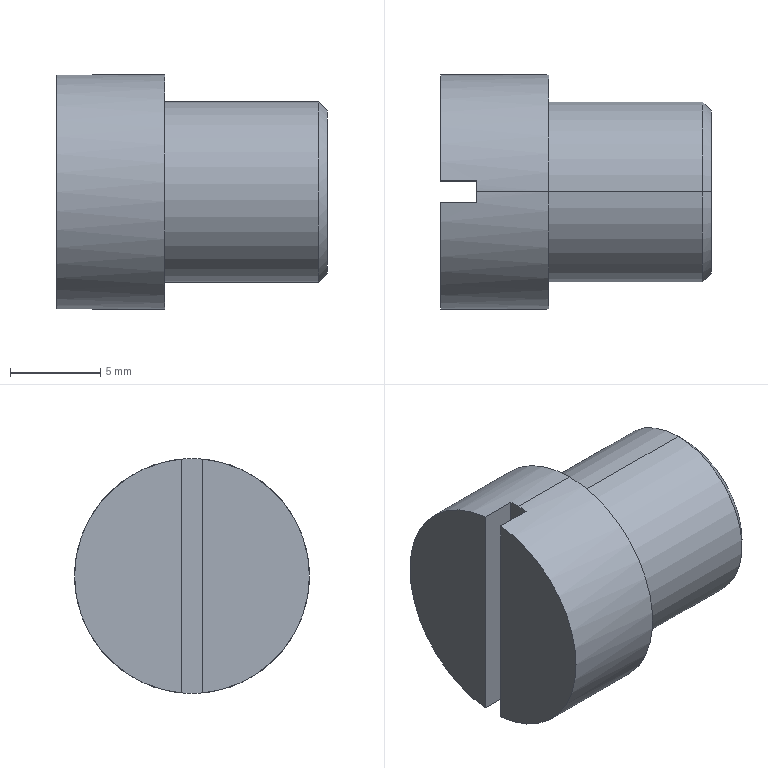Part | SolidWorks | features ICE 2, 3DProfileFeature 1, Chamfer 1, Extrusion 1, HoleWzd 1 | 1 solid | 17 faces | box 15 x 13 x 13 mm | volume 1310 mm3 | plane 7 | cylinder 6 | cone 4 | commonest cylinder face diameters 4.2 x2 10 x2 13 x2
STEP:
#1=CARTESIAN_POINT('',(9.,0.,-4.5));
#2=VERTEX_POINT('',#1);
#3=CARTESIAN_POINT('',(9.,0.,4.5));
#4=VERTEX_POINT('',#3);
#5=CARTESIAN_POINT('',(9.,0.,0.));
#6=DIRECTION('',(1.,0.,0.));
#7=DIRECTION('',(0.,0.,-1.));
#8=AXIS2_PLACEMENT_3D('',#5,#6,#7);
#9=CIRCLE('',#8,4.5);
#10=EDGE_CURVE('',#2,#4,#9,.T.);
#11=ORIENTED_EDGE('',*,*,#10,.F.);
#12=CARTESIAN_POINT('',(8.5,0.,-5.));
#13=VERTEX_POINT('',#12);
#14=CARTESIAN_POINT('',(9.,0.,-4.5));
#15=DIRECTION('',(-0.7071,0.,-0.7071));
#16=VECTOR('',#15,1000.);
#17=LINE('',#14,#16);
#18=EDGE_CURVE('',#2,#13,#17,.T.);
#19=ORIENTED_EDGE('',*,*,#18,.T.);
#20=CARTESIAN_POINT('',(8.5,0.,5.));
#21=VERTEX_POINT('',#20);
#22=CARTESIAN_POINT('',(8.5,0.,0.));
#23=DIRECTION('',(-1.,0.,0.));
#24=DIRECTION('',(0.,0.,-1.));
#25=AXIS2_PLACEMENT_3D('',#22,#23,#24);
#26=CIRCLE('',#25,5.);
#27=EDGE_CURVE('',#21,#13,#26,.T.);
#28=ORIENTED_EDGE('',*,*,#27,.F.);
#29=CARTESIAN_POINT('',(9.,0.,4.5));
#30=DIRECTION('',(-0.7071,0.,0.7071));
#31=VECTOR('',#30,1000.);
#32=LINE('',#29,#31);
#33=EDGE_CURVE('',#4,#21,#32,.T.);
#34=ORIENTED_EDGE('',*,*,#33,.F.);
#35=EDGE_LOOP('',(#11,#19,#28,#34));
#36=FACE_OUTER_BOUND('',#35,.T.);
#37=CARTESIAN_POINT('',(9.,0.,0.));
#38=DIRECTION('',(-1.,0.,0.));
#39=DIRECTION('',(0.,0.,1.));
#40=AXIS2_PLACEMENT_3D('',#37,#38,#39);
#41=CONICAL_SURFACE('',#40,4.5,0.7854);
#42=ADVANCED_FACE('',(#36),#41,.T.);
#43=CARTESIAN_POINT('',(-2.,0.,2.1));
#44=VERTEX_POINT('',#43);
#45=CARTESIAN_POINT('',(-2.,0.,-2.1));
#46=VERTEX_POINT('',#45);
#47=CARTESIAN_POINT('',(-2.,0.,0.));
#48=DIRECTION('',(1.,0.,0.));
#49=DIRECTION('',(0.,0.,-1.));
#50=AXIS2_PLACEMENT_3D('',#47,#48,#49);
#51=CIRCLE('',#50,2.1);
#52=EDGE_CURVE('',#44,#46,#51,.T.);
#53=ORIENTED_EDGE('',*,*,#52,.F.);
#54=CARTESIAN_POINT('',(9.,0.,2.1));
#55=VERTEX_POINT('',#54);
#56=CARTESIAN_POINT('',(9.,0.,2.1));
#57=DIRECTION('',(1.,0.,0.));
#58=VECTOR('',#57,1000.);
#59=LINE('',#56,#58);
#60=EDGE_CURVE('',#44,#55,#59,.T.);
#61=ORIENTED_EDGE('',*,*,#60,.T.);
#62=CARTESIAN_POINT('',(9.,0.,-2.1));
#63=VERTEX_POINT('',#62);
#64=CARTESIAN_POINT('',(9.,0.,0.));
#65=DIRECTION('',(1.,0.,0.));
#66=DIRECTION('',(0.,0.,-1.));
#67=AXIS2_PLACEMENT_3D('',#64,#65,#66);
#68=CIRCLE('',#67,2.1);
#69=EDGE_CURVE('',#55,#63,#68,.T.);
#70=ORIENTED_EDGE('',*,*,#69,.T.);
#71=CARTESIAN_POINT('',(9.,0.,-2.1));
#72=DIRECTION('',(1.,0.,0.));
#73=VECTOR('',#72,1000.);
#74=LINE('',#71,#73);
#75=EDGE_CURVE('',#46,#63,#74,.T.);
#76=ORIENTED_EDGE('',*,*,#75,.F.);
#77=EDGE_LOOP('',(#53,#61,#70,#76));
#78=FACE_OUTER_BOUND('',#77,.T.);
#79=CARTESIAN_POINT('',(9.,0.,0.));
#80=DIRECTION('',(1.,0.,0.));
#81=DIRECTION('',(0.,0.,-1.));
#82=AXIS2_PLACEMENT_3D('',#79,#80,#81);
#83=CYLINDRICAL_SURFACE('',#82,2.1);
#84=ADVANCED_FACE('',(#78),#83,.F.);
#85=CARTESIAN_POINT('',(-3.262,0.,0.));
#86=VERTEX_POINT('',#85);
#87=CARTESIAN_POINT('',(-2.,0.,-2.1));
#88=DIRECTION('',(0.515,0.,-0.8572));
#89=VECTOR('',#88,1000.);
#90=LINE('',#87,#89);
#91=EDGE_CURVE('',#86,#46,#90,.T.);
#92=ORIENTED_EDGE('',*,*,#91,.F.);
#93=CARTESIAN_POINT('',(-2.,0.,2.1));
#94=DIRECTION('',(0.515,0.,0.8572));
#95=VECTOR('',#94,1000.);
#96=LINE('',#93,#95);
#97=EDGE_CURVE('',#86,#44,#96,.T.);
#98=ORIENTED_EDGE('',*,*,#97,.T.);
#99=ORIENTED_EDGE('',*,*,#52,.T.);
#100=EDGE_LOOP('',(#92,#98,#99));
#101=FACE_OUTER_BOUND('',#100,.T.);
#102=CARTESIAN_POINT('',(-2.,0.,0.));
#103=DIRECTION('',(1.,0.,0.));
#104=DIRECTION('',(0.,0.,-1.));
#105=AXIS2_PLACEMENT_3D('',#102,#103,#104);
#106=CONICAL_SURFACE('',#105,2.1,1.03);
#107=ADVANCED_FACE('',(#101),#106,.F.);
#108=CARTESIAN_POINT('',(-4.,0.,6.5));
#109=VERTEX_POINT('',#108);
#110=CARTESIAN_POINT('',(-4.,0.6,6.472));
#111=VERTEX_POINT('',#110);
#112=CARTESIAN_POINT('',(-4.,0.,0.));
#113=DIRECTION('',(-1.,0.,0.));
#114=DIRECTION('',(0.,0.,1.));
#115=AXIS2_PLACEMENT_3D('',#112,#113,#114);
#116=CIRCLE('',#115,6.5);
#117=EDGE_CURVE('',#109,#111,#116,.T.);
#118=ORIENTED_EDGE('',*,*,#117,.F.);
#119=CARTESIAN_POINT('',(0.,0.,6.5));
#120=VERTEX_POINT('',#119);
#121=CARTESIAN_POINT('',(-6.,0.,6.5));
#122=DIRECTION('',(1.,0.,0.));
#123=VECTOR('',#122,1000.);
#124=LINE('',#121,#123);
#125=EDGE_CURVE('',#109,#120,#124,.T.);
#126=ORIENTED_EDGE('',*,*,#125,.T.);
#127=CARTESIAN_POINT('',(0.,0.,-6.5));
#128=VERTEX_POINT('',#127);
#129=CARTESIAN_POINT('',(0.,0.,0.));
#130=DIRECTION('',(-1.,0.,0.));
#131=DIRECTION('',(0.,0.,1.));
#132=AXIS2_PLACEMENT_3D('',#129,#130,#131);
#133=CIRCLE('',#132,6.5);
#134=EDGE_CURVE('',#120,#128,#133,.T.);
#135=ORIENTED_EDGE('',*,*,#134,.T.);
#136=CARTESIAN_POINT('',(-4.,0.,-6.5));
#137=VERTEX_POINT('',#136);
#138=CARTESIAN_POINT('',(-6.,0.,-6.5));
#139=DIRECTION('',(1.,0.,0.));
#140=VECTOR('',#139,1000.);
#141=LINE('',#138,#140);
#142=EDGE_CURVE('',#137,#128,#141,.T.);
#143=ORIENTED_EDGE('',*,*,#142,.F.);
#144=CARTESIAN_POINT('',(-4.,0.6,-6.472));
#145=VERTEX_POINT('',#144);
#146=CARTESIAN_POINT('',(-4.,0.,0.));
#147=DIRECTION('',(-1.,0.,0.));
#148=DIRECTION('',(0.,0.,1.));
#149=AXIS2_PLACEMENT_3D('',#146,#147,#148);
#150=CIRCLE('',#149,6.5);
#151=EDGE_CURVE('',#145,#137,#150,.T.);
#152=ORIENTED_EDGE('',*,*,#151,.F.);
#153=CARTESIAN_POINT('',(-6.,0.6,-6.472));
#154=VERTEX_POINT('',#153);
#155=CARTESIAN_POINT('',(-6.,0.6,-6.472));
#156=DIRECTION('',(-1.,0.,0.));
#157=VECTOR('',#156,1000.);
#158=LINE('',#155,#157);
#159=EDGE_CURVE('',#145,#154,#158,.T.);
#160=ORIENTED_EDGE('',*,*,#159,.T.);
#161=CARTESIAN_POINT('',(-6.,0.6,6.472));
#162=VERTEX_POINT('',#161);
#163=CARTESIAN_POINT('',(-6.,0.,0.));
#164=DIRECTION('',(-1.,0.,0.));
#165=DIRECTION('',(0.,0.,1.));
#166=AXIS2_PLACEMENT_3D('',#163,#164,#165);
#167=CIRCLE('',#166,6.5);
#168=EDGE_CURVE('',#162,#154,#167,.T.);
#169=ORIENTED_EDGE('',*,*,#168,.F.);
#170=CARTESIAN_POINT('',(-6.,0.6,6.472));
#171=DIRECTION('',(1.,0.,0.));
#172=VECTOR('',#171,1000.);
#173=LINE('',#170,#172);
#174=EDGE_CURVE('',#162,#111,#173,.T.);
#175=ORIENTED_EDGE('',*,*,#174,.T.);
#176=EDGE_LOOP('',(#118,#126,#135,#143,#152,#160,#169,#175));
#177=FACE_OUTER_BOUND('',#176,.T.);
#178=CARTESIAN_POINT('',(-6.,0.,0.));
#179=DIRECTION('',(1.,0.,0.));
#180=DIRECTION('',(0.,0.,-1.));
#181=AXIS2_PLACEMENT_3D('',#178,#179,#180);
#182=CYLINDRICAL_SURFACE('',#181,6.5);
#183=ADVANCED_FACE('',(#177),#182,.T.);
#184=ORIENTED_EDGE('',*,*,#27,.T.);
#185=CARTESIAN_POINT('',(0.,0.,-5.));
#186=VERTEX_POINT('',#185);
#187=CARTESIAN_POINT('',(9.,0.,-5.));
#188=DIRECTION('',(-1.,0.,0.));
#189=VECTOR('',#188,1000.);
#190=LINE('',#187,#189);
#191=EDGE_CURVE('',#13,#186,#190,.T.);
#192=ORIENTED_EDGE('',*,*,#191,.T.);
#193=CARTESIAN_POINT('',(0.,0.,5.));
#194=VERTEX_POINT('',#193);
#195=CARTESIAN_POINT('',(0.,0.,0.));
#196=DIRECTION('',(-1.,0.,0.));
#197=DIRECTION('',(0.,0.,1.));
#198=AXIS2_PLACEMENT_3D('',#195,#196,#197);
#199=CIRCLE('',#198,5.);
#200=EDGE_CURVE('',#194,#186,#199,.T.);
#201=ORIENTED_EDGE('',*,*,#200,.F.);
#202=CARTESIAN_POINT('',(9.,0.,5.));
#203=DIRECTION('',(-1.,0.,0.));
#204=VECTOR('',#203,1000.);
#205=LINE('',#202,#204);
#206=EDGE_CURVE('',#21,#194,#205,.T.);
#207=ORIENTED_EDGE('',*,*,#206,.F.);
#208=EDGE_LOOP('',(#184,#192,#201,#207));
#209=FACE_OUTER_BOUND('',#208,.T.);
#210=CARTESIAN_POINT('',(9.,0.,0.));
#211=DIRECTION('',(-1.,0.,0.));
#212=DIRECTION('',(0.,0.,1.));
#213=AXIS2_PLACEMENT_3D('',#210,#211,#212);
#214=CYLINDRICAL_SURFACE('',#213,5.);
#215=ADVANCED_FACE('',(#209),#214,.T.);
#216=CARTESIAN_POINT('',(-6.,-0.6,-6.472));
#217=VERTEX_POINT('',#216);
#218=CARTESIAN_POINT('',(-6.,-0.6,6.472));
#219=VERTEX_POINT('',#218);
#220=CARTESIAN_POINT('',(-6.,-0.6,0.));
#221=DIRECTION('',(0.,0.,1.));
#222=VECTOR('',#221,1000.);
#223=LINE('',#220,#222);
#224=EDGE_CURVE('',#217,#219,#223,.T.);
#225=ORIENTED_EDGE('',*,*,#224,.F.);
#226=CARTESIAN_POINT('',(-6.,0.,0.));
#227=DIRECTION('',(-1.,0.,0.));
#228=DIRECTION('',(0.,0.,1.));
#229=AXIS2_PLACEMENT_3D('',#226,#227,#228);
#230=CIRCLE('',#229,6.5);
#231=EDGE_CURVE('',#217,#219,#230,.T.);
#232=ORIENTED_EDGE('',*,*,#231,.T.);
#233=EDGE_LOOP('',(#225,#232));
#234=FACE_OUTER_BOUND('',#233,.T.);
#235=CARTESIAN_POINT('',(-6.,0.,0.));
#236=DIRECTION('',(-1.,0.,0.));
#237=DIRECTION('',(0.,0.,1.));
#238=AXIS2_PLACEMENT_3D('',#235,#236,#237);
#239=PLANE('',#238);
#240=ADVANCED_FACE('',(#234),#239,.T.);
#241=ORIENTED_EDGE('',*,*,#191,.F.);
#242=CARTESIAN_POINT('',(8.5,0.,0.));
#243=DIRECTION('',(-1.,0.,0.));
#244=DIRECTION('',(0.,0.,-1.));
#245=AXIS2_PLACEMENT_3D('',#242,#243,#244);
#246=CIRCLE('',#245,5.);
#247=EDGE_CURVE('',#13,#21,#246,.T.);
#248=ORIENTED_EDGE('',*,*,#247,.T.);
#249=ORIENTED_EDGE('',*,*,#206,.T.);
#250=CARTESIAN_POINT('',(0.,0.,0.));
#251=DIRECTION('',(-1.,0.,0.));
#252=DIRECTION('',(0.,0.,1.));
#253=AXIS2_PLACEMENT_3D('',#250,#251,#252);
#254=CIRCLE('',#253,5.);
#255=EDGE_CURVE('',#186,#194,#254,.T.);
#256=ORIENTED_EDGE('',*,*,#255,.F.);
#257=EDGE_LOOP('',(#241,#248,#249,#256));
#258=FACE_OUTER_BOUND('',#257,.T.);
#259=CARTESIAN_POINT('',(9.,0.,0.));
#260=DIRECTION('',(-1.,0.,0.));
#261=DIRECTION('',(0.,0.,1.));
#262=AXIS2_PLACEMENT_3D('',#259,#260,#261);
#263=CYLINDRICAL_SURFACE('',#262,5.);
#264=ADVANCED_FACE('',(#258),#263,.T.);
#265=CARTESIAN_POINT('',(9.,0.,0.));
#266=DIRECTION('',(1.,0.,0.));
#267=DIRECTION('',(0.,0.,-1.));
#268=AXIS2_PLACEMENT_3D('',#265,#266,#267);
#269=CIRCLE('',#268,4.5);
#270=EDGE_CURVE('',#4,#2,#269,.T.);
#271=ORIENTED_EDGE('',*,*,#270,.T.);
#272=ORIENTED_EDGE('',*,*,#10,.T.);
#273=EDGE_LOOP('',(#271,#272));
#274=FACE_OUTER_BOUND('',#273,.T.);
#275=CARTESIAN_POINT('',(9.,0.,0.));
#276=DIRECTION('',(1.,0.,0.));
#277=DIRECTION('',(0.,0.,-1.));
#278=AXIS2_PLACEMENT_3D('',#275,#276,#277);
#279=CIRCLE('',#278,2.1);
#280=EDGE_CURVE('',#63,#55,#279,.T.);
#281=ORIENTED_EDGE('',*,*,#280,.F.);
#282=ORIENTED_EDGE('',*,*,#69,.F.);
#283=EDGE_LOOP('',(#281,#282));
#284=FACE_BOUND('',#283,.T.);
#285=CARTESIAN_POINT('',(9.,0.,0.));
#286=DIRECTION('',(1.,0.,0.));
#287=DIRECTION('',(0.,0.,-1.));
#288=AXIS2_PLACEMENT_3D('',#285,#286,#287);
#289=PLANE('',#288);
#290=ADVANCED_FACE('',(#274,#284),#289,.T.);
#291=CARTESIAN_POINT('',(0.,0.,0.));
#292=DIRECTION('',(-1.,0.,0.));
#293=DIRECTION('',(0.,0.,1.));
#294=AXIS2_PLACEMENT_3D('',#291,#292,#293);
#295=CIRCLE('',#294,6.5);
#296=EDGE_CURVE('',#128,#120,#295,.T.);
#297=ORIENTED_EDGE('',*,*,#296,.F.);
#298=ORIENTED_EDGE('',*,*,#134,.F.);
#299=EDGE_LOOP('',(#297,#298));
#300=FACE_OUTER_BOUND('',#299,.T.);
#301=ORIENTED_EDGE('',*,*,#200,.T.);
#302=ORIENTED_EDGE('',*,*,#255,.T.);
#303=EDGE_LOOP('',(#301,#302));
#304=FACE_BOUND('',#303,.T.);
#305=CARTESIAN_POINT('',(0.,0.,0.));
#306=DIRECTION('',(-1.,0.,0.));
#307=DIRECTION('',(0.,0.,1.));
#308=AXIS2_PLACEMENT_3D('',#305,#306,#307);
#309=PLANE('',#308);
#310=ADVANCED_FACE('',(#300,#304),#309,.F.);
#311=ORIENTED_EDGE('',*,*,#125,.F.);
#312=CARTESIAN_POINT('',(-4.,-0.6,6.472));
#313=VERTEX_POINT('',#312);
#314=CARTESIAN_POINT('',(-4.,0.,0.));
#315=DIRECTION('',(-1.,0.,0.));
#316=DIRECTION('',(0.,0.,1.));
#317=AXIS2_PLACEMENT_3D('',#314,#315,#316);
#318=CIRCLE('',#317,6.5);
#319=EDGE_CURVE('',#313,#109,#318,.T.);
#320=ORIENTED_EDGE('',*,*,#319,.F.);
#321=CARTESIAN_POINT('',(-6.,-0.6,6.472));
#322=DIRECTION('',(-1.,0.,0.));
#323=VECTOR('',#322,1000.);
#324=LINE('',#321,#323);
#325=EDGE_CURVE('',#313,#219,#324,.T.);
#326=ORIENTED_EDGE('',*,*,#325,.T.);
#327=ORIENTED_EDGE('',*,*,#231,.F.);
#328=CARTESIAN_POINT('',(-4.,-0.6,-6.472));
#329=VERTEX_POINT('',#328);
#330=CARTESIAN_POINT('',(-6.,-0.6,-6.472));
#331=DIRECTION('',(1.,0.,0.));
#332=VECTOR('',#331,1000.);
#333=LINE('',#330,#332);
#334=EDGE_CURVE('',#217,#329,#333,.T.);
#335=ORIENTED_EDGE('',*,*,#334,.T.);
#336=CARTESIAN_POINT('',(-4.,0.,0.));
#337=DIRECTION('',(-1.,0.,0.));
#338=DIRECTION('',(0.,0.,1.));
#339=AXIS2_PLACEMENT_3D('',#336,#337,#338);
#340=CIRCLE('',#339,6.5);
#341=EDGE_CURVE('',#137,#329,#340,.T.);
#342=ORIENTED_EDGE('',*,*,#341,.F.);
#343=ORIENTED_EDGE('',*,*,#142,.T.);
#344=ORIENTED_EDGE('',*,*,#296,.T.);
#345=EDGE_LOOP('',(#311,#320,#326,#327,#335,#342,#343,#344));
#346=FACE_OUTER_BOUND('',#345,.T.);
#347=CARTESIAN_POINT('',(-6.,0.,0.));
#348=DIRECTION('',(1.,0.,0.));
#349=DIRECTION('',(0.,0.,-1.));
#350=AXIS2_PLACEMENT_3D('',#347,#348,#349);
#351=CYLINDRICAL_SURFACE('',#350,6.5);
#352=ADVANCED_FACE('',(#346),#351,.T.);
#353=CARTESIAN_POINT('',(-6.,0.6,0.));
#354=DIRECTION('',(0.,0.,-1.));
#355=VECTOR('',#354,1000.);
#356=LINE('',#353,#355);
#357=EDGE_CURVE('',#162,#154,#356,.T.);
#358=ORIENTED_EDGE('',*,*,#357,.F.);
#359=ORIENTED_EDGE('',*,*,#168,.T.);
#360=EDGE_LOOP('',(#358,#359));
#361=FACE_OUTER_BOUND('',#360,.T.);
#362=CARTESIAN_POINT('',(-6.,0.,0.));
#363=DIRECTION('',(-1.,0.,0.));
#364=DIRECTION('',(0.,0.,1.));
#365=AXIS2_PLACEMENT_3D('',#362,#363,#364);
#366=PLANE('',#365);
#367=ADVANCED_FACE('',(#361),#366,.T.);
#368=ORIENTED_EDGE('',*,*,#151,.T.);
#369=ORIENTED_EDGE('',*,*,#341,.T.);
#370=CARTESIAN_POINT('',(-4.,-0.6,-15.));
#371=DIRECTION('',(0.,0.,1.));
#372=VECTOR('',#371,1000.);
#373=LINE('',#370,#372);
#374=EDGE_CURVE('',#329,#313,#373,.T.);
#375=ORIENTED_EDGE('',*,*,#374,.T.);
#376=ORIENTED_EDGE('',*,*,#319,.T.);
#377=ORIENTED_EDGE('',*,*,#117,.T.);
#378=CARTESIAN_POINT('',(-4.,0.6,-15.));
#379=DIRECTION('',(0.,0.,-1.));
#380=VECTOR('',#379,1000.);
#381=LINE('',#378,#380);
#382=EDGE_CURVE('',#111,#145,#381,.T.);
#383=ORIENTED_EDGE('',*,*,#382,.T.);
#384=EDGE_LOOP('',(#368,#369,#375,#376,#377,#383));
#385=FACE_OUTER_BOUND('',#384,.T.);
#386=CARTESIAN_POINT('',(-4.,0.,0.));
#387=DIRECTION('',(-1.,0.,0.));
#388=DIRECTION('',(0.,0.,1.));
#389=AXIS2_PLACEMENT_3D('',#386,#387,#388);
#390=PLANE('',#389);
#391=ADVANCED_FACE('',(#385),#390,.T.);
#392=ORIENTED_EDGE('',*,*,#224,.T.);
#393=ORIENTED_EDGE('',*,*,#325,.F.);
#394=ORIENTED_EDGE('',*,*,#374,.F.);
#395=ORIENTED_EDGE('',*,*,#334,.F.);
#396=EDGE_LOOP('',(#392,#393,#394,#395));
#397=FACE_OUTER_BOUND('',#396,.T.);
#398=CARTESIAN_POINT('',(-4.,-0.6,-15.));
#399=DIRECTION('',(0.,-1.,0.));
#400=DIRECTION('',(0.,0.,-1.));
#401=AXIS2_PLACEMENT_3D('',#398,#399,#400);
#402=PLANE('',#401);
#403=ADVANCED_FACE('',(#397),#402,.F.);
#404=ORIENTED_EDGE('',*,*,#357,.T.);
#405=ORIENTED_EDGE('',*,*,#159,.F.);
#406=ORIENTED_EDGE('',*,*,#382,.F.);
#407=ORIENTED_EDGE('',*,*,#174,.F.);
#408=EDGE_LOOP('',(#404,#405,#406,#407));
#409=FACE_OUTER_BOUND('',#408,.T.);
#410=CARTESIAN_POINT('',(-4.,0.6,-15.));
#411=DIRECTION('',(0.,1.,0.));
#412=DIRECTION('',(0.,0.,1.));
#413=AXIS2_PLACEMENT_3D('',#410,#411,#412);
#414=PLANE('',#413);
#415=ADVANCED_FACE('',(#409),#414,.F.);
#416=ORIENTED_EDGE('',*,*,#97,.F.);
#417=ORIENTED_EDGE('',*,*,#91,.T.);
#418=CARTESIAN_POINT('',(-2.,0.,0.));
#419=DIRECTION('',(1.,0.,0.));
#420=DIRECTION('',(0.,0.,-1.));
#421=AXIS2_PLACEMENT_3D('',#418,#419,#420);
#422=CIRCLE('',#421,2.1);
#423=EDGE_CURVE('',#46,#44,#422,.T.);
#424=ORIENTED_EDGE('',*,*,#423,.T.);
#425=EDGE_LOOP('',(#416,#417,#424));
#426=FACE_OUTER_BOUND('',#425,.T.);
#427=CARTESIAN_POINT('',(-2.,0.,0.));
#428=DIRECTION('',(1.,0.,0.));
#429=DIRECTION('',(0.,0.,-1.));
#430=AXIS2_PLACEMENT_3D('',#427,#428,#429);
#431=CONICAL_SURFACE('',#430,2.1,1.03);
#432=ADVANCED_FACE('',(#426),#431,.F.);
#433=ORIENTED_EDGE('',*,*,#60,.F.);
#434=ORIENTED_EDGE('',*,*,#423,.F.);
#435=ORIENTED_EDGE('',*,*,#75,.T.);
#436=ORIENTED_EDGE('',*,*,#280,.T.);
#437=EDGE_LOOP('',(#433,#434,#435,#436));
#438=FACE_OUTER_BOUND('',#437,.T.);
#439=CARTESIAN_POINT('',(9.,0.,0.));
#440=DIRECTION('',(1.,0.,0.));
#441=DIRECTION('',(0.,0.,-1.));
#442=AXIS2_PLACEMENT_3D('',#439,#440,#441);
#443=CYLINDRICAL_SURFACE('',#442,2.1);
#444=ADVANCED_FACE('',(#438),#443,.F.);
#445=ORIENTED_EDGE('',*,*,#18,.F.);
#446=ORIENTED_EDGE('',*,*,#270,.F.);
#447=ORIENTED_EDGE('',*,*,#33,.T.);
#448=ORIENTED_EDGE('',*,*,#247,.F.);
#449=EDGE_LOOP('',(#445,#446,#447,#448));
#450=FACE_OUTER_BOUND('',#449,.T.);
#451=CARTESIAN_POINT('',(9.,0.,0.));
#452=DIRECTION('',(-1.,0.,0.));
#453=DIRECTION('',(0.,0.,1.));
#454=AXIS2_PLACEMENT_3D('',#451,#452,#453);
#455=CONICAL_SURFACE('',#454,4.5,0.7854);
#456=ADVANCED_FACE('',(#450),#455,.T.);
#457=CLOSED_SHELL('',(#42,#84,#107,#183,#215,#240,#264,#290,#310,#352,#367,#391,#403,#415,#432,#444,#456));
#458=MANIFOLD_SOLID_BREP('',#457);
#459=CARTESIAN_POINT('',(0.,0.,0.));
#460=DIRECTION('',(0.,0.,1.));
#461=DIRECTION('',(1.,0.,0.));
#462=AXIS2_PLACEMENT_3D('',#459,#460,#461);
#463=(LENGTH_UNIT()NAMED_UNIT(*)SI_UNIT(.MILLI.,.METRE.));
#464=UNCERTAINTY_MEASURE_WITH_UNIT(LENGTH_MEASURE(0.00001),#463,'','');
#465=(NAMED_UNIT(*)PLANE_ANGLE_UNIT()SI_UNIT($,.RADIAN.));
#466=(NAMED_UNIT(*)SI_UNIT($,.STERADIAN.)SOLID_ANGLE_UNIT());
#467=(GEOMETRIC_REPRESENTATION_CONTEXT(3)GLOBAL_UNCERTAINTY_ASSIGNED_CONTEXT((#464))GLOBAL_UNIT_ASSIGNED_CONTEXT((#463,#465,#466))REPRESENTATION_CONTEXT('',''));
#468=ADVANCED_BREP_SHAPE_REPRESENTATION('',(#458,#462),#467);